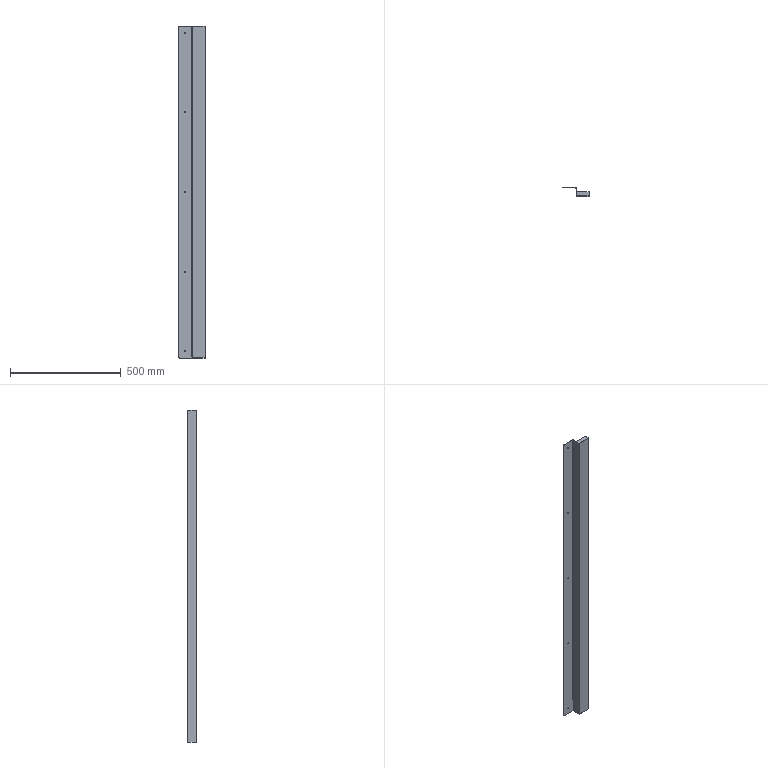Part | SolidWorks | features ICE 4, ExtruThin 1, Fillet 1, FlatPattern 1, FlattenBends 1, ProcessBends 1, SheetMetal 1 | 1 solid | 62 faces | box 120 x 40 x 1500 mm | volume 161482 mm3 | plane 40 | cylinder 22 | commonest cylinder face diameters 5.5 x10 0.6 x5 1.8 x5 10 x2